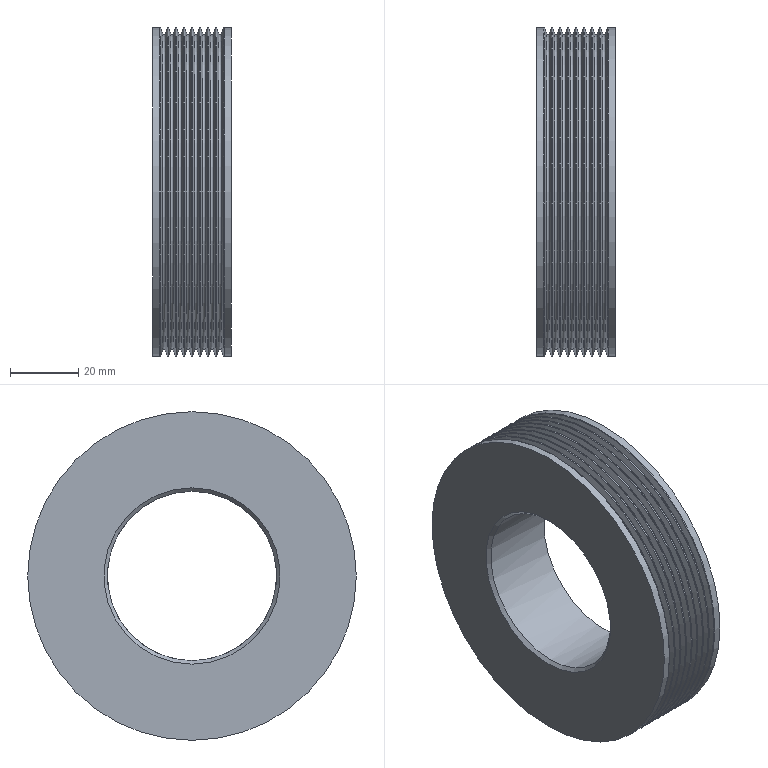Part | STEP file | PN_0019_default | 1 solid | 41 faces | box 23 x 96 x 96 mm | volume 114860 mm3 | torus 17 | cone 17 | cylinder 4 | plane 3 | commonest cylinder face diameters 96 x2 13 x1 49.5 x1